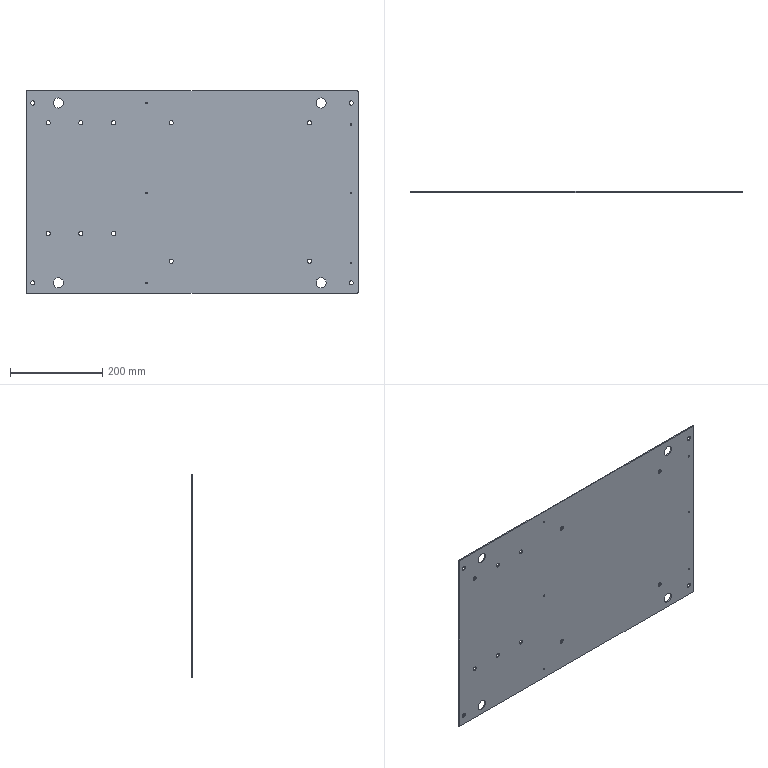Part | NX | features solid 2 | 1 solid | 58 faces | box 720 x 2.5 x 440 mm | volume 785768 mm3 | cylinder 52 | plane 6 | commonest cylinder face diameters 9.2 x20 3.242 x12 9 x8 22 x8 4 x4